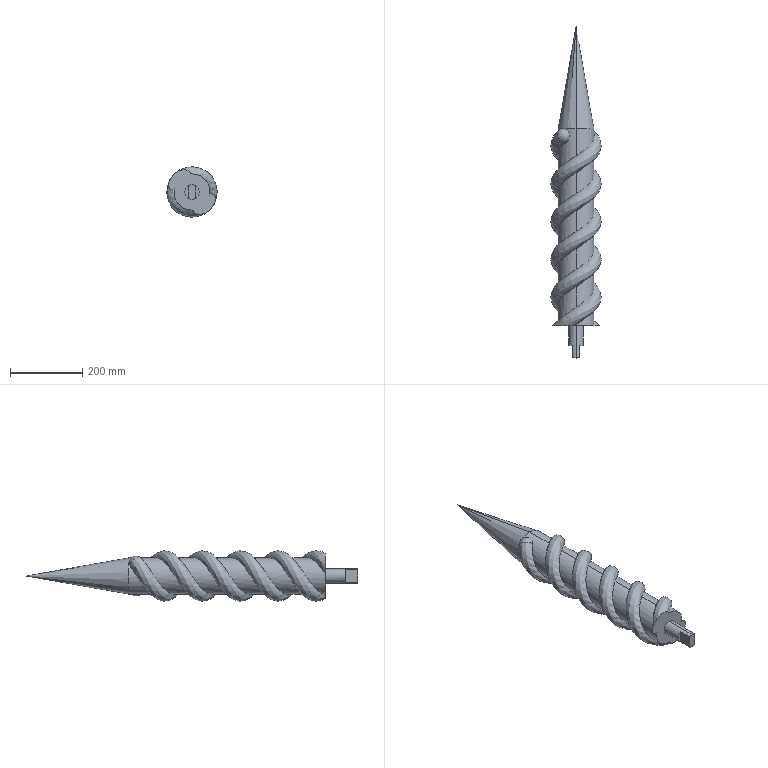Part | SolidWorks | 1 solid | 26 faces | volume 6506170 mm3 | cylinder 14 | plane 6 | cone 2 | spline 2 | sphere 2 | commonest cylinder face diameters 100 x12 40 x2